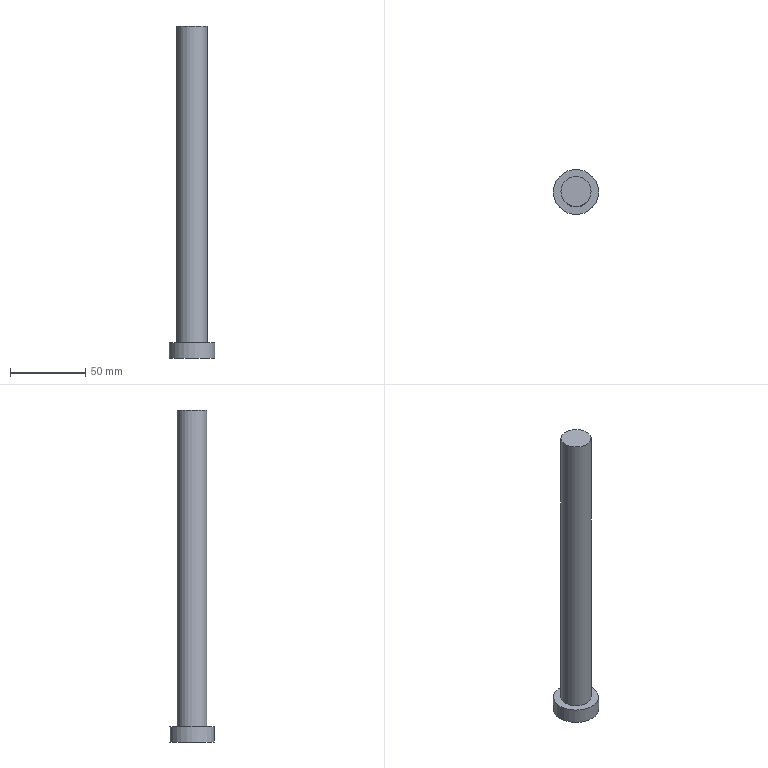Part | NX | features 护邦千斤顶滑块销 2 | 1 solid | 5 faces | box 30 x 30 x 220 mm | volume 73042 mm3 | plane 3 | cylinder 2 | commonest cylinder face diameters 20 x1 30 x1
STEP:
#1=CARTESIAN_POINT('',(10.,0.,210.));
#2=VERTEX_POINT('',#1);
#3=CARTESIAN_POINT('',(0.,0.,210.));
#4=DIRECTION('',(0.,0.,1.));
#5=DIRECTION('',(1.,0.,0.));
#6=AXIS2_PLACEMENT_3D('',#3,#4,#5);
#7=CIRCLE('',#6,10.);
#8=EDGE_CURVE('',#2,#2,#7,.T.);
#9=ORIENTED_EDGE('',*,*,#8,.F.);
#10=EDGE_LOOP('',(#9));
#11=FACE_BOUND('',#10,.T.);
#12=CARTESIAN_POINT('',(-10.,0.,0.));
#13=VERTEX_POINT('',#12);
#14=CARTESIAN_POINT('',(0.,0.,0.));
#15=DIRECTION('',(0.,0.,-1.));
#16=DIRECTION('',(-1.,0.,0.));
#17=AXIS2_PLACEMENT_3D('',#14,#15,#16);
#18=CIRCLE('',#17,10.);
#19=EDGE_CURVE('',#13,#13,#18,.T.);
#20=ORIENTED_EDGE('',*,*,#19,.F.);
#21=EDGE_LOOP('',(#20));
#22=FACE_BOUND('',#21,.T.);
#23=CARTESIAN_POINT('',(0.,0.,210.));
#24=DIRECTION('',(0.,0.,-1.));
#25=DIRECTION('',(-1.,0.,0.));
#26=AXIS2_PLACEMENT_3D('',#23,#24,#25);
#27=CYLINDRICAL_SURFACE('',#26,10.);
#28=ADVANCED_FACE('',(#11,#22),#27,.T.);
#29=ORIENTED_EDGE('',*,*,#8,.T.);
#30=EDGE_LOOP('',(#29));
#31=FACE_BOUND('',#30,.T.);
#32=CARTESIAN_POINT('',(0.,0.,210.));
#33=DIRECTION('',(0.,0.,1.));
#34=DIRECTION('',(1.,0.,0.));
#35=AXIS2_PLACEMENT_3D('',#32,#33,#34);
#36=PLANE('',#35);
#37=ADVANCED_FACE('',(#31),#36,.T.);
#38=CARTESIAN_POINT('',(-15.,0.,0.));
#39=VERTEX_POINT('',#38);
#40=CARTESIAN_POINT('',(0.,0.,0.));
#41=DIRECTION('',(0.,0.,-1.));
#42=DIRECTION('',(-1.,0.,0.));
#43=AXIS2_PLACEMENT_3D('',#40,#41,#42);
#44=CIRCLE('',#43,15.);
#45=EDGE_CURVE('',#39,#39,#44,.T.);
#46=ORIENTED_EDGE('',*,*,#45,.F.);
#47=EDGE_LOOP('',(#46));
#48=FACE_BOUND('',#47,.T.);
#49=ORIENTED_EDGE('',*,*,#19,.T.);
#50=EDGE_LOOP('',(#49));
#51=FACE_BOUND('',#50,.T.);
#52=CARTESIAN_POINT('',(0.,0.,0.));
#53=DIRECTION('',(0.,0.,-1.));
#54=DIRECTION('',(-1.,0.,0.));
#55=AXIS2_PLACEMENT_3D('',#52,#53,#54);
#56=PLANE('',#55);
#57=ADVANCED_FACE('',(#48,#51),#56,.F.);
#58=CARTESIAN_POINT('',(-15.,0.,-10.));
#59=VERTEX_POINT('',#58);
#60=CARTESIAN_POINT('',(0.,0.,-10.));
#61=DIRECTION('',(0.,0.,-1.));
#62=DIRECTION('',(-1.,0.,0.));
#63=AXIS2_PLACEMENT_3D('',#60,#61,#62);
#64=CIRCLE('',#63,15.);
#65=EDGE_CURVE('',#59,#59,#64,.T.);
#66=ORIENTED_EDGE('',*,*,#65,.F.);
#67=EDGE_LOOP('',(#66));
#68=FACE_BOUND('',#67,.T.);
#69=ORIENTED_EDGE('',*,*,#45,.T.);
#70=EDGE_LOOP('',(#69));
#71=FACE_BOUND('',#70,.T.);
#72=CARTESIAN_POINT('',(0.,0.,-10.));
#73=DIRECTION('',(0.,0.,1.));
#74=DIRECTION('',(1.,0.,0.));
#75=AXIS2_PLACEMENT_3D('',#72,#73,#74);
#76=CYLINDRICAL_SURFACE('',#75,15.);
#77=ADVANCED_FACE('',(#68,#71),#76,.T.);
#78=ORIENTED_EDGE('',*,*,#65,.T.);
#79=EDGE_LOOP('',(#78));
#80=FACE_BOUND('',#79,.T.);
#81=CARTESIAN_POINT('',(0.,0.,-10.));
#82=DIRECTION('',(0.,0.,-1.));
#83=DIRECTION('',(-1.,0.,0.));
#84=AXIS2_PLACEMENT_3D('',#81,#82,#83);
#85=PLANE('',#84);
#86=ADVANCED_FACE('',(#80),#85,.T.);
#87=CLOSED_SHELL('',(#28,#37,#57,#77,#86));
#88=MANIFOLD_SOLID_BREP('',#87);
#89=(LENGTH_UNIT()NAMED_UNIT(*)SI_UNIT(.MILLI.,.METRE.));
#90=UNCERTAINTY_MEASURE_WITH_UNIT(LENGTH_MEASURE(0.00001),#89,'','');
#91=(NAMED_UNIT(*)PLANE_ANGLE_UNIT()SI_UNIT($,.RADIAN.));
#92=(NAMED_UNIT(*)SI_UNIT($,.STERADIAN.)SOLID_ANGLE_UNIT());
#93=(GEOMETRIC_REPRESENTATION_CONTEXT(3)GLOBAL_UNCERTAINTY_ASSIGNED_CONTEXT((#90))GLOBAL_UNIT_ASSIGNED_CONTEXT((#89,#91,#92))REPRESENTATION_CONTEXT('',''));
#94=ADVANCED_BREP_SHAPE_REPRESENTATION('',(#88),#93);